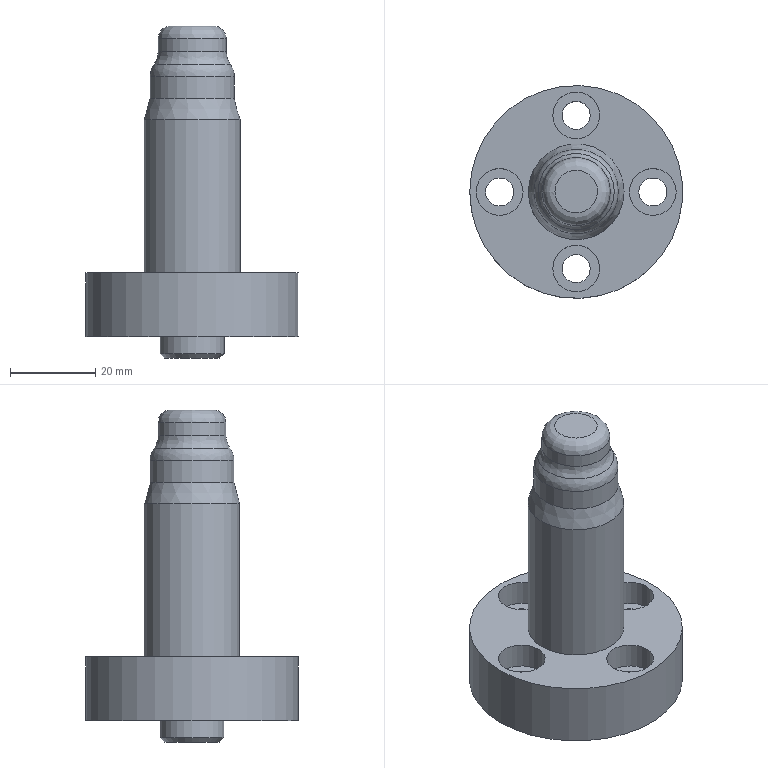Part | NX | features mandrel expand 2 | 1 solid | 26 faces | box 50 x 50 x 78 mm | volume 47044 mm3 | cylinder 13 | plane 8 | spline 3 | cone 2 | commonest cylinder face diameters 6.6 x4 11 x4 15 x1 16 x1 19.8 x1 22.5 x1